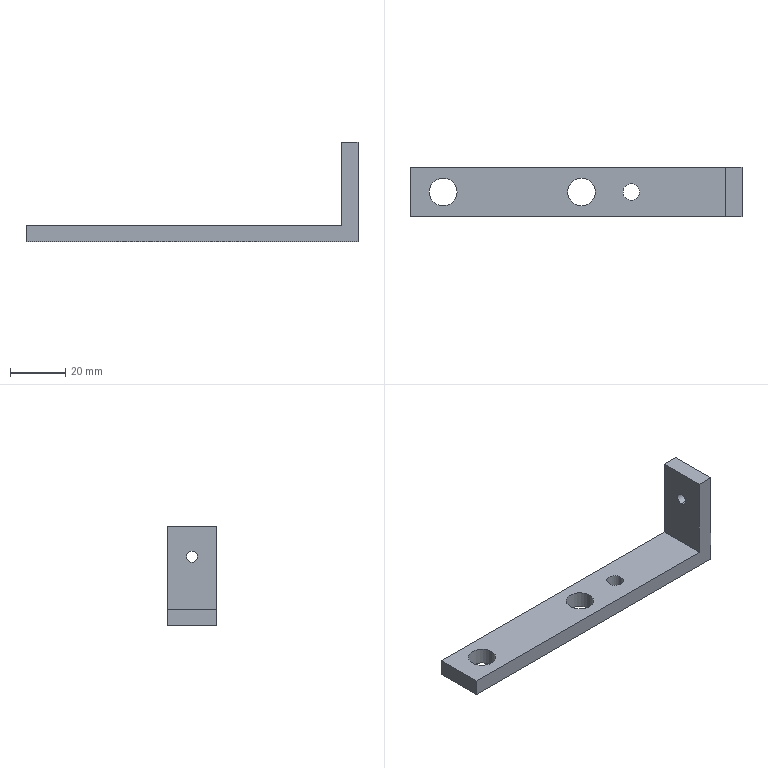Part | SolidWorks | features ICE 5, Extrusion 1 | 1 solid | 16 faces | box 120 x 18 x 36 mm | volume 15012 mm3 | cylinder 8 | plane 8 | commonest cylinder face diameters 10 x4 4 x2 6 x2
STEP:
#1=CARTESIAN_POINT('',(66.5,0.,27.));
#2=VERTEX_POINT('',#1);
#3=CARTESIAN_POINT('',(66.5,0.,23.));
#4=VERTEX_POINT('',#3);
#5=CARTESIAN_POINT('',(66.5,0.,25.));
#6=DIRECTION('',(1.,0.,0.));
#7=DIRECTION('',(0.,0.,-1.));
#8=AXIS2_PLACEMENT_3D('',#5,#6,#7);
#9=CIRCLE('',#8,2.);
#10=EDGE_CURVE('',#2,#4,#9,.T.);
#11=ORIENTED_EDGE('',*,*,#10,.F.);
#12=CARTESIAN_POINT('',(72.5,0.,27.));
#13=VERTEX_POINT('',#12);
#14=CARTESIAN_POINT('',(52.5,0.,27.));
#15=DIRECTION('',(1.,0.,0.));
#16=VECTOR('',#15,1000.);
#17=LINE('',#14,#16);
#18=EDGE_CURVE('',#2,#13,#17,.T.);
#19=ORIENTED_EDGE('',*,*,#18,.T.);
#20=CARTESIAN_POINT('',(72.5,0.,23.));
#21=VERTEX_POINT('',#20);
#22=CARTESIAN_POINT('',(72.5,0.,25.));
#23=DIRECTION('',(1.,0.,0.));
#24=DIRECTION('',(0.,0.,-1.));
#25=AXIS2_PLACEMENT_3D('',#22,#23,#24);
#26=CIRCLE('',#25,2.);
#27=EDGE_CURVE('',#13,#21,#26,.T.);
#28=ORIENTED_EDGE('',*,*,#27,.T.);
#29=CARTESIAN_POINT('',(52.5,0.,23.));
#30=DIRECTION('',(1.,0.,0.));
#31=VECTOR('',#30,1000.);
#32=LINE('',#29,#31);
#33=EDGE_CURVE('',#4,#21,#32,.T.);
#34=ORIENTED_EDGE('',*,*,#33,.F.);
#35=EDGE_LOOP('',(#11,#19,#28,#34));
#36=FACE_OUTER_BOUND('',#35,.T.);
#37=CARTESIAN_POINT('',(52.5,0.,25.));
#38=DIRECTION('',(1.,0.,0.));
#39=DIRECTION('',(0.,0.,-1.));
#40=AXIS2_PLACEMENT_3D('',#37,#38,#39);
#41=CYLINDRICAL_SURFACE('',#40,2.);
#42=ADVANCED_FACE('',(#36),#41,.F.);
#43=CARTESIAN_POINT('',(35.5,0.,6.));
#44=VERTEX_POINT('',#43);
#45=CARTESIAN_POINT('',(29.5,0.,6.));
#46=VERTEX_POINT('',#45);
#47=CARTESIAN_POINT('',(32.5,0.,6.));
#48=DIRECTION('',(0.,0.,-1.));
#49=DIRECTION('',(-1.,0.,0.));
#50=AXIS2_PLACEMENT_3D('',#47,#48,#49);
#51=CIRCLE('',#50,3.);
#52=EDGE_CURVE('',#44,#46,#51,.T.);
#53=ORIENTED_EDGE('',*,*,#52,.F.);
#54=CARTESIAN_POINT('',(35.5,0.,0.));
#55=VERTEX_POINT('',#54);
#56=CARTESIAN_POINT('',(35.5,0.,10.));
#57=DIRECTION('',(0.,0.,-1.));
#58=VECTOR('',#57,1000.);
#59=LINE('',#56,#58);
#60=EDGE_CURVE('',#44,#55,#59,.T.);
#61=ORIENTED_EDGE('',*,*,#60,.T.);
#62=CARTESIAN_POINT('',(29.5,0.,0.));
#63=VERTEX_POINT('',#62);
#64=CARTESIAN_POINT('',(32.5,0.,0.));
#65=DIRECTION('',(0.,0.,-1.));
#66=DIRECTION('',(-1.,0.,0.));
#67=AXIS2_PLACEMENT_3D('',#64,#65,#66);
#68=CIRCLE('',#67,3.);
#69=EDGE_CURVE('',#55,#63,#68,.T.);
#70=ORIENTED_EDGE('',*,*,#69,.T.);
#71=CARTESIAN_POINT('',(29.5,0.,10.));
#72=DIRECTION('',(0.,0.,-1.));
#73=VECTOR('',#72,1000.);
#74=LINE('',#71,#73);
#75=EDGE_CURVE('',#46,#63,#74,.T.);
#76=ORIENTED_EDGE('',*,*,#75,.F.);
#77=EDGE_LOOP('',(#53,#61,#70,#76));
#78=FACE_OUTER_BOUND('',#77,.T.);
#79=CARTESIAN_POINT('',(32.5,0.,10.));
#80=DIRECTION('',(0.,0.,-1.));
#81=DIRECTION('',(-1.,0.,0.));
#82=AXIS2_PLACEMENT_3D('',#79,#80,#81);
#83=CYLINDRICAL_SURFACE('',#82,3.);
#84=ADVANCED_FACE('',(#78),#83,.F.);
#85=CARTESIAN_POINT('',(9.5,0.,0.));
#86=VERTEX_POINT('',#85);
#87=CARTESIAN_POINT('',(19.5,0.,0.));
#88=VERTEX_POINT('',#87);
#89=CARTESIAN_POINT('',(14.5,0.,0.));
#90=DIRECTION('',(0.,0.,1.));
#91=DIRECTION('',(1.,0.,0.));
#92=AXIS2_PLACEMENT_3D('',#89,#90,#91);
#93=CIRCLE('',#92,5.);
#94=EDGE_CURVE('',#86,#88,#93,.T.);
#95=ORIENTED_EDGE('',*,*,#94,.F.);
#96=CARTESIAN_POINT('',(9.5,0.,6.));
#97=VERTEX_POINT('',#96);
#98=CARTESIAN_POINT('',(9.5,0.,0.));
#99=DIRECTION('',(0.,0.,1.));
#100=VECTOR('',#99,1000.);
#101=LINE('',#98,#100);
#102=EDGE_CURVE('',#86,#97,#101,.T.);
#103=ORIENTED_EDGE('',*,*,#102,.T.);
#104=CARTESIAN_POINT('',(19.5,0.,6.));
#105=VERTEX_POINT('',#104);
#106=CARTESIAN_POINT('',(14.5,0.,6.));
#107=DIRECTION('',(0.,0.,1.));
#108=DIRECTION('',(1.,0.,0.));
#109=AXIS2_PLACEMENT_3D('',#106,#107,#108);
#110=CIRCLE('',#109,5.);
#111=EDGE_CURVE('',#97,#105,#110,.T.);
#112=ORIENTED_EDGE('',*,*,#111,.T.);
#113=CARTESIAN_POINT('',(19.5,0.,0.));
#114=DIRECTION('',(0.,0.,1.));
#115=VECTOR('',#114,1000.);
#116=LINE('',#113,#115);
#117=EDGE_CURVE('',#88,#105,#116,.T.);
#118=ORIENTED_EDGE('',*,*,#117,.F.);
#119=EDGE_LOOP('',(#95,#103,#112,#118));
#120=FACE_OUTER_BOUND('',#119,.T.);
#121=CARTESIAN_POINT('',(14.5,0.,0.));
#122=DIRECTION('',(0.,0.,1.));
#123=DIRECTION('',(1.,0.,0.));
#124=AXIS2_PLACEMENT_3D('',#121,#122,#123);
#125=CYLINDRICAL_SURFACE('',#124,5.);
#126=ADVANCED_FACE('',(#120),#125,.F.);
#127=CARTESIAN_POINT('',(-40.5,0.,0.));
#128=VERTEX_POINT('',#127);
#129=CARTESIAN_POINT('',(-30.5,0.,0.));
#130=VERTEX_POINT('',#129);
#131=CARTESIAN_POINT('',(-35.5,0.,0.));
#132=DIRECTION('',(0.,0.,1.));
#133=DIRECTION('',(1.,0.,0.));
#134=AXIS2_PLACEMENT_3D('',#131,#132,#133);
#135=CIRCLE('',#134,5.);
#136=EDGE_CURVE('',#128,#130,#135,.T.);
#137=ORIENTED_EDGE('',*,*,#136,.F.);
#138=CARTESIAN_POINT('',(-40.5,0.,6.));
#139=VERTEX_POINT('',#138);
#140=CARTESIAN_POINT('',(-40.5,0.,0.));
#141=DIRECTION('',(0.,0.,1.));
#142=VECTOR('',#141,1000.);
#143=LINE('',#140,#142);
#144=EDGE_CURVE('',#128,#139,#143,.T.);
#145=ORIENTED_EDGE('',*,*,#144,.T.);
#146=CARTESIAN_POINT('',(-30.5,0.,6.));
#147=VERTEX_POINT('',#146);
#148=CARTESIAN_POINT('',(-35.5,0.,6.));
#149=DIRECTION('',(0.,0.,1.));
#150=DIRECTION('',(1.,0.,0.));
#151=AXIS2_PLACEMENT_3D('',#148,#149,#150);
#152=CIRCLE('',#151,5.);
#153=EDGE_CURVE('',#139,#147,#152,.T.);
#154=ORIENTED_EDGE('',*,*,#153,.T.);
#155=CARTESIAN_POINT('',(-30.5,0.,0.));
#156=DIRECTION('',(0.,0.,1.));
#157=VECTOR('',#156,1000.);
#158=LINE('',#155,#157);
#159=EDGE_CURVE('',#130,#147,#158,.T.);
#160=ORIENTED_EDGE('',*,*,#159,.F.);
#161=EDGE_LOOP('',(#137,#145,#154,#160));
#162=FACE_OUTER_BOUND('',#161,.T.);
#163=CARTESIAN_POINT('',(-35.5,0.,0.));
#164=DIRECTION('',(0.,0.,1.));
#165=DIRECTION('',(1.,0.,0.));
#166=AXIS2_PLACEMENT_3D('',#163,#164,#165);
#167=CYLINDRICAL_SURFACE('',#166,5.);
#168=ADVANCED_FACE('',(#162),#167,.F.);
#169=CARTESIAN_POINT('',(-35.5,0.,6.));
#170=DIRECTION('',(0.,0.,1.));
#171=DIRECTION('',(1.,0.,0.));
#172=AXIS2_PLACEMENT_3D('',#169,#170,#171);
#173=CIRCLE('',#172,5.);
#174=EDGE_CURVE('',#147,#139,#173,.T.);
#175=ORIENTED_EDGE('',*,*,#174,.F.);
#176=ORIENTED_EDGE('',*,*,#153,.F.);
#177=EDGE_LOOP('',(#175,#176));
#178=FACE_BOUND('',#177,.T.);
#179=CARTESIAN_POINT('',(14.5,0.,6.));
#180=DIRECTION('',(0.,0.,1.));
#181=DIRECTION('',(1.,0.,0.));
#182=AXIS2_PLACEMENT_3D('',#179,#180,#181);
#183=CIRCLE('',#182,5.);
#184=EDGE_CURVE('',#105,#97,#183,.T.);
#185=ORIENTED_EDGE('',*,*,#184,.F.);
#186=ORIENTED_EDGE('',*,*,#111,.F.);
#187=EDGE_LOOP('',(#185,#186));
#188=FACE_BOUND('',#187,.T.);
#189=CARTESIAN_POINT('',(32.5,0.,6.));
#190=DIRECTION('',(0.,0.,-1.));
#191=DIRECTION('',(-1.,0.,0.));
#192=AXIS2_PLACEMENT_3D('',#189,#190,#191);
#193=CIRCLE('',#192,3.);
#194=EDGE_CURVE('',#46,#44,#193,.T.);
#195=ORIENTED_EDGE('',*,*,#194,.T.);
#196=ORIENTED_EDGE('',*,*,#52,.T.);
#197=EDGE_LOOP('',(#195,#196));
#198=FACE_BOUND('',#197,.T.);
#199=CARTESIAN_POINT('',(66.5,9.,6.));
#200=VERTEX_POINT('',#199);
#201=CARTESIAN_POINT('',(66.5,-9.,6.));
#202=VERTEX_POINT('',#201);
#203=CARTESIAN_POINT('',(66.5,9.,6.));
#204=DIRECTION('',(0.,-1.,0.));
#205=VECTOR('',#204,1000.);
#206=LINE('',#203,#205);
#207=EDGE_CURVE('',#200,#202,#206,.T.);
#208=ORIENTED_EDGE('',*,*,#207,.F.);
#209=CARTESIAN_POINT('',(-47.5,9.,6.));
#210=VERTEX_POINT('',#209);
#211=CARTESIAN_POINT('',(-47.5,9.,6.));
#212=DIRECTION('',(-1.,0.,0.));
#213=VECTOR('',#212,1000.);
#214=LINE('',#211,#213);
#215=EDGE_CURVE('',#200,#210,#214,.T.);
#216=ORIENTED_EDGE('',*,*,#215,.T.);
#217=CARTESIAN_POINT('',(-47.5,-9.,6.));
#218=VERTEX_POINT('',#217);
#219=CARTESIAN_POINT('',(-47.5,-9.,6.));
#220=DIRECTION('',(0.,-1.,0.));
#221=VECTOR('',#220,1000.);
#222=LINE('',#219,#221);
#223=EDGE_CURVE('',#210,#218,#222,.T.);
#224=ORIENTED_EDGE('',*,*,#223,.T.);
#225=CARTESIAN_POINT('',(-47.5,-9.,6.));
#226=DIRECTION('',(1.,0.,0.));
#227=VECTOR('',#226,1000.);
#228=LINE('',#225,#227);
#229=EDGE_CURVE('',#218,#202,#228,.T.);
#230=ORIENTED_EDGE('',*,*,#229,.T.);
#231=EDGE_LOOP('',(#208,#216,#224,#230));
#232=FACE_OUTER_BOUND('',#231,.T.);
#233=CARTESIAN_POINT('',(0.,0.,6.));
#234=DIRECTION('',(0.,0.,-1.));
#235=DIRECTION('',(-1.,0.,0.));
#236=AXIS2_PLACEMENT_3D('',#233,#234,#235);
#237=PLANE('',#236);
#238=ADVANCED_FACE('',(#178,#188,#198,#232),#237,.F.);
#239=CARTESIAN_POINT('',(72.5,9.,0.));
#240=VERTEX_POINT('',#239);
#241=CARTESIAN_POINT('',(-47.5,9.,0.));
#242=VERTEX_POINT('',#241);
#243=CARTESIAN_POINT('',(-47.5,9.,0.));
#244=DIRECTION('',(-1.,0.,0.));
#245=VECTOR('',#244,1000.);
#246=LINE('',#243,#245);
#247=EDGE_CURVE('',#240,#242,#246,.T.);
#248=ORIENTED_EDGE('',*,*,#247,.T.);
#249=CARTESIAN_POINT('',(-47.5,9.,6.));
#250=DIRECTION('',(0.,0.,-1.));
#251=VECTOR('',#250,1000.);
#252=LINE('',#249,#251);
#253=EDGE_CURVE('',#210,#242,#252,.T.);
#254=ORIENTED_EDGE('',*,*,#253,.F.);
#255=ORIENTED_EDGE('',*,*,#215,.F.);
#256=CARTESIAN_POINT('',(66.5,9.,36.));
#257=VERTEX_POINT('',#256);
#258=CARTESIAN_POINT('',(66.5,9.,36.));
#259=DIRECTION('',(0.,0.,-1.));
#260=VECTOR('',#259,1000.);
#261=LINE('',#258,#260);
#262=EDGE_CURVE('',#257,#200,#261,.T.);
#263=ORIENTED_EDGE('',*,*,#262,.F.);
#264=CARTESIAN_POINT('',(72.5,9.,36.));
#265=VERTEX_POINT('',#264);
#266=CARTESIAN_POINT('',(72.5,9.,36.));
#267=DIRECTION('',(-1.,0.,0.));
#268=VECTOR('',#267,1000.);
#269=LINE('',#266,#268);
#270=EDGE_CURVE('',#265,#257,#269,.T.);
#271=ORIENTED_EDGE('',*,*,#270,.F.);
#272=CARTESIAN_POINT('',(72.5,9.,0.));
#273=DIRECTION('',(0.,0.,1.));
#274=VECTOR('',#273,1000.);
#275=LINE('',#272,#274);
#276=EDGE_CURVE('',#240,#265,#275,.T.);
#277=ORIENTED_EDGE('',*,*,#276,.F.);
#278=EDGE_LOOP('',(#248,#254,#255,#263,#271,#277));
#279=FACE_OUTER_BOUND('',#278,.T.);
#280=CARTESIAN_POINT('',(-47.5,9.,6.));
#281=DIRECTION('',(0.,-1.,0.));
#282=DIRECTION('',(0.,0.,-1.));
#283=AXIS2_PLACEMENT_3D('',#280,#281,#282);
#284=PLANE('',#283);
#285=ADVANCED_FACE('',(#279),#284,.F.);
#286=CARTESIAN_POINT('',(-47.5,-9.,0.));
#287=VERTEX_POINT('',#286);
#288=CARTESIAN_POINT('',(-47.5,-9.,0.));
#289=DIRECTION('',(0.,-1.,0.));
#290=VECTOR('',#289,1000.);
#291=LINE('',#288,#290);
#292=EDGE_CURVE('',#242,#287,#291,.T.);
#293=ORIENTED_EDGE('',*,*,#292,.T.);
#294=CARTESIAN_POINT('',(-47.5,-9.,6.));
#295=DIRECTION('',(0.,0.,-1.));
#296=VECTOR('',#295,1000.);
#297=LINE('',#294,#296);
#298=EDGE_CURVE('',#218,#287,#297,.T.);
#299=ORIENTED_EDGE('',*,*,#298,.F.);
#300=ORIENTED_EDGE('',*,*,#223,.F.);
#301=ORIENTED_EDGE('',*,*,#253,.T.);
#302=EDGE_LOOP('',(#293,#299,#300,#301));
#303=FACE_OUTER_BOUND('',#302,.T.);
#304=CARTESIAN_POINT('',(-47.5,-9.,6.));
#305=DIRECTION('',(1.,0.,0.));
#306=DIRECTION('',(0.,0.,-1.));
#307=AXIS2_PLACEMENT_3D('',#304,#305,#306);
#308=PLANE('',#307);
#309=ADVANCED_FACE('',(#303),#308,.F.);
#310=CARTESIAN_POINT('',(72.5,-9.,0.));
#311=VERTEX_POINT('',#310);
#312=CARTESIAN_POINT('',(-47.5,-9.,0.));
#313=DIRECTION('',(1.,0.,0.));
#314=VECTOR('',#313,1000.);
#315=LINE('',#312,#314);
#316=EDGE_CURVE('',#287,#311,#315,.T.);
#317=ORIENTED_EDGE('',*,*,#316,.T.);
#318=CARTESIAN_POINT('',(72.5,-9.,36.));
#319=VERTEX_POINT('',#318);
#320=CARTESIAN_POINT('',(72.5,-9.,0.));
#321=DIRECTION('',(0.,0.,-1.));
#322=VECTOR('',#321,1000.);
#323=LINE('',#320,#322);
#324=EDGE_CURVE('',#319,#311,#323,.T.);
#325=ORIENTED_EDGE('',*,*,#324,.F.);
#326=CARTESIAN_POINT('',(66.5,-9.,36.));
#327=VERTEX_POINT('',#326);
#328=CARTESIAN_POINT('',(72.5,-9.,36.));
#329=DIRECTION('',(1.,0.,0.));
#330=VECTOR('',#329,1000.);
#331=LINE('',#328,#330);
#332=EDGE_CURVE('',#327,#319,#331,.T.);
#333=ORIENTED_EDGE('',*,*,#332,.F.);
#334=CARTESIAN_POINT('',(66.5,-9.,36.));
#335=DIRECTION('',(0.,0.,-1.));
#336=VECTOR('',#335,1000.);
#337=LINE('',#334,#336);
#338=EDGE_CURVE('',#327,#202,#337,.T.);
#339=ORIENTED_EDGE('',*,*,#338,.T.);
#340=ORIENTED_EDGE('',*,*,#229,.F.);
#341=ORIENTED_EDGE('',*,*,#298,.T.);
#342=EDGE_LOOP('',(#317,#325,#333,#339,#340,#341));
#343=FACE_OUTER_BOUND('',#342,.T.);
#344=CARTESIAN_POINT('',(-47.5,-9.,6.));
#345=DIRECTION('',(0.,1.,0.));
#346=DIRECTION('',(0.,0.,1.));
#347=AXIS2_PLACEMENT_3D('',#344,#345,#346);
#348=PLANE('',#347);
#349=ADVANCED_FACE('',(#343),#348,.F.);
#350=CARTESIAN_POINT('',(32.5,0.,0.));
#351=DIRECTION('',(0.,0.,-1.));
#352=DIRECTION('',(-1.,0.,0.));
#353=AXIS2_PLACEMENT_3D('',#350,#351,#352);
#354=CIRCLE('',#353,3.);
#355=EDGE_CURVE('',#63,#55,#354,.T.);
#356=ORIENTED_EDGE('',*,*,#355,.F.);
#357=ORIENTED_EDGE('',*,*,#69,.F.);
#358=EDGE_LOOP('',(#356,#357));
#359=FACE_BOUND('',#358,.T.);
#360=CARTESIAN_POINT('',(14.5,0.,0.));
#361=DIRECTION('',(0.,0.,1.));
#362=DIRECTION('',(1.,0.,0.));
#363=AXIS2_PLACEMENT_3D('',#360,#361,#362);
#364=CIRCLE('',#363,5.);
#365=EDGE_CURVE('',#88,#86,#364,.T.);
#366=ORIENTED_EDGE('',*,*,#365,.T.);
#367=ORIENTED_EDGE('',*,*,#94,.T.);
#368=EDGE_LOOP('',(#366,#367));
#369=FACE_BOUND('',#368,.T.);
#370=CARTESIAN_POINT('',(-35.5,0.,0.));
#371=DIRECTION('',(0.,0.,1.));
#372=DIRECTION('',(1.,0.,0.));
#373=AXIS2_PLACEMENT_3D('',#370,#371,#372);
#374=CIRCLE('',#373,5.);
#375=EDGE_CURVE('',#130,#128,#374,.T.);
#376=ORIENTED_EDGE('',*,*,#375,.T.);
#377=ORIENTED_EDGE('',*,*,#136,.T.);
#378=EDGE_LOOP('',(#376,#377));
#379=FACE_BOUND('',#378,.T.);
#380=ORIENTED_EDGE('',*,*,#247,.F.);
#381=CARTESIAN_POINT('',(72.5,9.,0.));
#382=DIRECTION('',(0.,1.,0.));
#383=VECTOR('',#382,1000.);
#384=LINE('',#381,#383);
#385=EDGE_CURVE('',#311,#240,#384,.T.);
#386=ORIENTED_EDGE('',*,*,#385,.F.);
#387=ORIENTED_EDGE('',*,*,#316,.F.);
#388=ORIENTED_EDGE('',*,*,#292,.F.);
#389=EDGE_LOOP('',(#380,#386,#387,#388));
#390=FACE_OUTER_BOUND('',#389,.T.);
#391=CARTESIAN_POINT('',(0.,0.,0.));
#392=DIRECTION('',(0.,0.,-1.));
#393=DIRECTION('',(-1.,0.,0.));
#394=AXIS2_PLACEMENT_3D('',#391,#392,#393);
#395=PLANE('',#394);
#396=ADVANCED_FACE('',(#359,#369,#379,#390),#395,.T.);
#397=ORIENTED_EDGE('',*,*,#144,.F.);
#398=ORIENTED_EDGE('',*,*,#375,.F.);
#399=ORIENTED_EDGE('',*,*,#159,.T.);
#400=ORIENTED_EDGE('',*,*,#174,.T.);
#401=EDGE_LOOP('',(#397,#398,#399,#400));
#402=FACE_OUTER_BOUND('',#401,.T.);
#403=CARTESIAN_POINT('',(-35.5,0.,0.));
#404=DIRECTION('',(0.,0.,1.));
#405=DIRECTION('',(1.,0.,0.));
#406=AXIS2_PLACEMENT_3D('',#403,#404,#405);
#407=CYLINDRICAL_SURFACE('',#406,5.);
#408=ADVANCED_FACE('',(#402),#407,.F.);
#409=ORIENTED_EDGE('',*,*,#102,.F.);
#410=ORIENTED_EDGE('',*,*,#365,.F.);
#411=ORIENTED_EDGE('',*,*,#117,.T.);
#412=ORIENTED_EDGE('',*,*,#184,.T.);
#413=EDGE_LOOP('',(#409,#410,#411,#412));
#414=FACE_OUTER_BOUND('',#413,.T.);
#415=CARTESIAN_POINT('',(14.5,0.,0.));
#416=DIRECTION('',(0.,0.,1.));
#417=DIRECTION('',(1.,0.,0.));
#418=AXIS2_PLACEMENT_3D('',#415,#416,#417);
#419=CYLINDRICAL_SURFACE('',#418,5.);
#420=ADVANCED_FACE('',(#414),#419,.F.);
#421=ORIENTED_EDGE('',*,*,#60,.F.);
#422=ORIENTED_EDGE('',*,*,#194,.F.);
#423=ORIENTED_EDGE('',*,*,#75,.T.);
#424=ORIENTED_EDGE('',*,*,#355,.T.);
#425=EDGE_LOOP('',(#421,#422,#423,#424));
#426=FACE_OUTER_BOUND('',#425,.T.);
#427=CARTESIAN_POINT('',(32.5,0.,10.));
#428=DIRECTION('',(0.,0.,-1.));
#429=DIRECTION('',(-1.,0.,0.));
#430=AXIS2_PLACEMENT_3D('',#427,#428,#429);
#431=CYLINDRICAL_SURFACE('',#430,3.);
#432=ADVANCED_FACE('',(#426),#431,.F.);
#433=CARTESIAN_POINT('',(72.5,0.,25.));
#434=DIRECTION('',(1.,0.,0.));
#435=DIRECTION('',(0.,0.,-1.));
#436=AXIS2_PLACEMENT_3D('',#433,#434,#435);
#437=CIRCLE('',#436,2.);
#438=EDGE_CURVE('',#21,#13,#437,.T.);
#439=ORIENTED_EDGE('',*,*,#438,.F.);
#440=ORIENTED_EDGE('',*,*,#27,.F.);
#441=EDGE_LOOP('',(#439,#440));
#442=FACE_BOUND('',#441,.T.);
#443=ORIENTED_EDGE('',*,*,#385,.T.);
#444=ORIENTED_EDGE('',*,*,#276,.T.);
#445=CARTESIAN_POINT('',(72.5,9.,36.));
#446=DIRECTION('',(0.,1.,0.));
#447=VECTOR('',#446,1000.);
#448=LINE('',#445,#447);
#449=EDGE_CURVE('',#319,#265,#448,.T.);
#450=ORIENTED_EDGE('',*,*,#449,.F.);
#451=ORIENTED_EDGE('',*,*,#324,.T.);
#452=EDGE_LOOP('',(#443,#444,#450,#451));
#453=FACE_OUTER_BOUND('',#452,.T.);
#454=CARTESIAN_POINT('',(72.5,0.,0.));
#455=DIRECTION('',(-1.,0.,0.));
#456=DIRECTION('',(0.,0.,1.));
#457=AXIS2_PLACEMENT_3D('',#454,#455,#456);
#458=PLANE('',#457);
#459=ADVANCED_FACE('',(#442,#453),#458,.F.);
#460=CARTESIAN_POINT('',(66.5,0.,25.));
#461=DIRECTION('',(1.,0.,0.));
#462=DIRECTION('',(0.,0.,-1.));
#463=AXIS2_PLACEMENT_3D('',#460,#461,#462);
#464=CIRCLE('',#463,2.);
#465=EDGE_CURVE('',#4,#2,#464,.T.);
#466=ORIENTED_EDGE('',*,*,#465,.T.);
#467=ORIENTED_EDGE('',*,*,#10,.T.);
#468=EDGE_LOOP('',(#466,#467));
#469=FACE_BOUND('',#468,.T.);
#470=ORIENTED_EDGE('',*,*,#207,.T.);
#471=ORIENTED_EDGE('',*,*,#338,.F.);
#472=CARTESIAN_POINT('',(66.5,9.,36.));
#473=DIRECTION('',(0.,-1.,0.));
#474=VECTOR('',#473,1000.);
#475=LINE('',#472,#474);
#476=EDGE_CURVE('',#257,#327,#475,.T.);
#477=ORIENTED_EDGE('',*,*,#476,.F.);
#478=ORIENTED_EDGE('',*,*,#262,.T.);
#479=EDGE_LOOP('',(#470,#471,#477,#478));
#480=FACE_OUTER_BOUND('',#479,.T.);
#481=CARTESIAN_POINT('',(66.5,9.,36.));
#482=DIRECTION('',(1.,0.,0.));
#483=DIRECTION('',(0.,0.,-1.));
#484=AXIS2_PLACEMENT_3D('',#481,#482,#483);
#485=PLANE('',#484);
#486=ADVANCED_FACE('',(#469,#480),#485,.F.);
#487=ORIENTED_EDGE('',*,*,#449,.T.);
#488=ORIENTED_EDGE('',*,*,#270,.T.);
#489=ORIENTED_EDGE('',*,*,#476,.T.);
#490=ORIENTED_EDGE('',*,*,#332,.T.);
#491=EDGE_LOOP('',(#487,#488,#489,#490));
#492=FACE_OUTER_BOUND('',#491,.T.);
#493=CARTESIAN_POINT('',(0.,0.,36.));
#494=DIRECTION('',(0.,0.,-1.));
#495=DIRECTION('',(-1.,0.,0.));
#496=AXIS2_PLACEMENT_3D('',#493,#494,#495);
#497=PLANE('',#496);
#498=ADVANCED_FACE('',(#492),#497,.F.);
#499=ORIENTED_EDGE('',*,*,#18,.F.);
#500=ORIENTED_EDGE('',*,*,#465,.F.);
#501=ORIENTED_EDGE('',*,*,#33,.T.);
#502=ORIENTED_EDGE('',*,*,#438,.T.);
#503=EDGE_LOOP('',(#499,#500,#501,#502));
#504=FACE_OUTER_BOUND('',#503,.T.);
#505=CARTESIAN_POINT('',(52.5,0.,25.));
#506=DIRECTION('',(1.,0.,0.));
#507=DIRECTION('',(0.,0.,-1.));
#508=AXIS2_PLACEMENT_3D('',#505,#506,#507);
#509=CYLINDRICAL_SURFACE('',#508,2.);
#510=ADVANCED_FACE('',(#504),#509,.F.);
#511=CLOSED_SHELL('',(#42,#84,#126,#168,#238,#285,#309,#349,#396,#408,#420,#432,#459,#486,#498,#510));
#512=MANIFOLD_SOLID_BREP('',#511);
#513=CARTESIAN_POINT('',(0.,0.,0.));
#514=DIRECTION('',(0.,0.,1.));
#515=DIRECTION('',(1.,0.,0.));
#516=AXIS2_PLACEMENT_3D('',#513,#514,#515);
#517=(LENGTH_UNIT()NAMED_UNIT(*)SI_UNIT(.MILLI.,.METRE.));
#518=UNCERTAINTY_MEASURE_WITH_UNIT(LENGTH_MEASURE(0.00001),#517,'','');
#519=(NAMED_UNIT(*)PLANE_ANGLE_UNIT()SI_UNIT($,.RADIAN.));
#520=(NAMED_UNIT(*)SI_UNIT($,.STERADIAN.)SOLID_ANGLE_UNIT());
#521=(GEOMETRIC_REPRESENTATION_CONTEXT(3)GLOBAL_UNCERTAINTY_ASSIGNED_CONTEXT((#518))GLOBAL_UNIT_ASSIGNED_CONTEXT((#517,#519,#520))REPRESENTATION_CONTEXT('',''));
#522=ADVANCED_BREP_SHAPE_REPRESENTATION('',(#512,#516),#521);